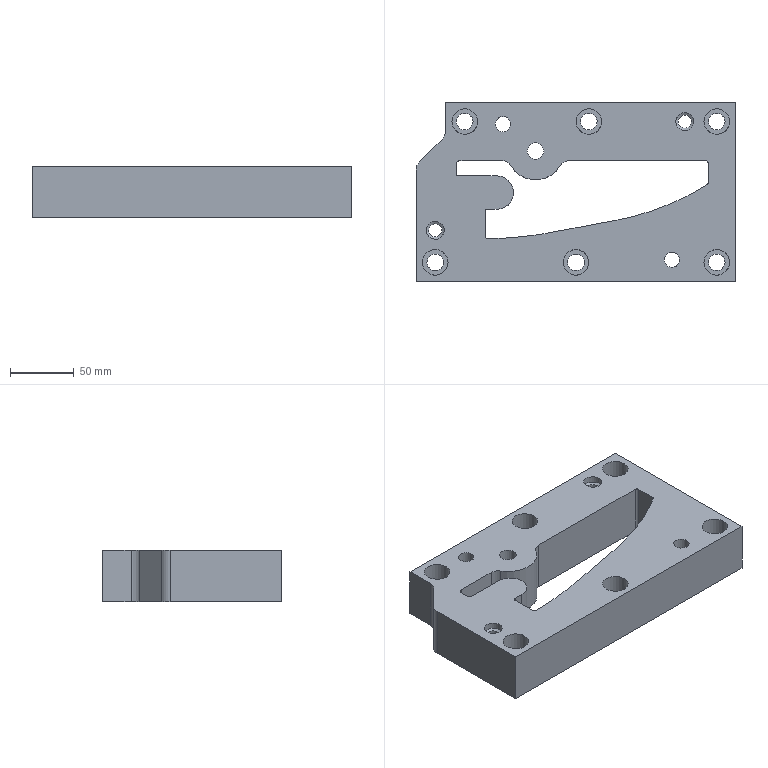Part | STEP file | gslz 2016.10.28-13_id486_x_t | 1 solid | 67 faces | box 250 x 140 x 40 mm | volume 992848 mm3 | cylinder 33 | plane 32 | cone 2 | commonest cylinder face diameters 13 x7 20 x6 4 x5 10.3 x2 12 x2 14 x2